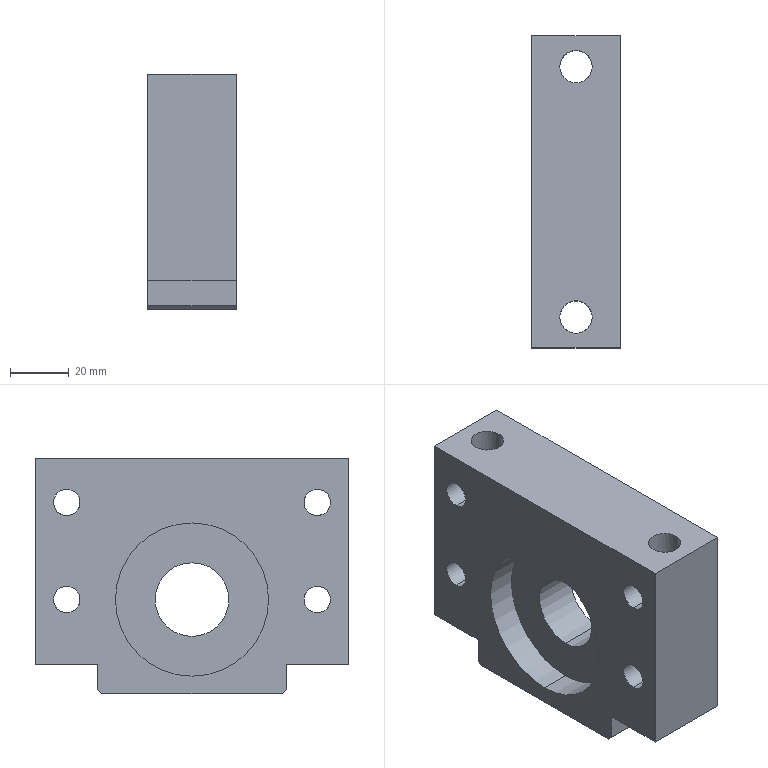Part | STEP file | bearing fixing block BF25 | 2 solids | 46 faces | box 30 x 106 x 80 mm | volume 180921 mm3 | cylinder 30 | plane 16 | commonest cylinder face diameters 9 x16 11 x4 17.5 x4 52 x4 25 x2